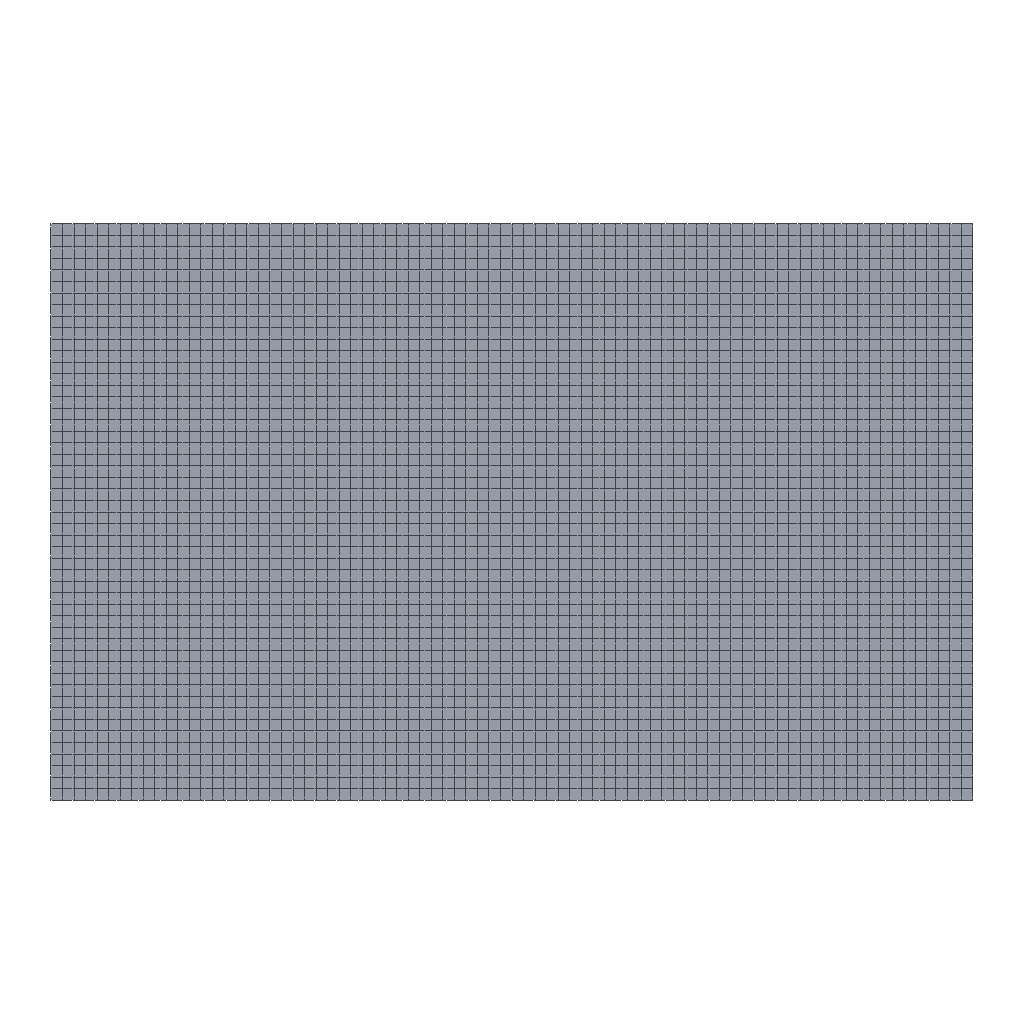Simulation study | abaqus
Set-up summary:
category,name,step,type,value,unit,region
solver,abaqus
solver,version,,,Abaqus/Standard 2020
units,not stated in the deck,,not stated
analysis,deck,,geostatic,geostatic
load_step,Step-1,Step-1,geostatic
load_step,Step-2,Step-2,soils
load_step,requested,,,2
mesh,nodes,,,4164
mesh,elements,,,4030
element_type,T2D2,,truss,30
element_type,CPE4P,,plane,4000
load,load commands in deck,,count,4
bc,support commands in deck,,count,3
material,CRACK,,in results
material,ROCK,,in results
check,setup vs results,,match,"per instance, exact: element labels, types and connectivity; labels of the nodes the elements use; coordinates of those nodes at SINGLE_PRECISION in 4 of 4 instance(s)"
Abaqus input file, long lists of numbers shortened:
*Heading
** Job name: Job-2 Model name: Model-1
** Generated by: Abaqus/CAE 2020
*Preprint, echo=NO, model=NO, history=NO, contact=NO
**
** PARTS
**
*Part, name=CRACK
*Node
      1,         -25.,          -4.
      2,         -25.,          -5.
** (9 more lines like these left out)
*Element, type=T2D2
 1,  1,  3
 2,  3,  4
** (8 more lines like these left out)
*Nset, nset=Set-1, generate
  1,  11,   1
*Elset, elset=Set-1, generate
  1,  10,   1
*Nset, nset=Set-4, generate
  1,  11,   1
*Elset, elset=Set-4, generate
  1,  10,   1
*Nset, nset=Set-5, generate
  1,  11,   1
*Elset, elset=Set-5, generate
  1,  10,   1
*Nset, nset=Set-14, generate
  1,  11,   1
*Elset, elset=Set-14, generate
  1,  10,   1
** Section: crack
*Solid Section, elset=Set-14, material=CRACK
1.,
*End Part
**
*Part, name=ROCK
*Node
      1,        58.75,        31.25
      2,        57.75,        31.25
** (4129 more lines like these left out)
*Element, type=CPE4P
   1,    1,    2,   83,   82
   2,    2,    3,   84,   83
** (3998 more lines like these left out)
*Nset, nset=Set-1, generate
    1,  4131,     1
*Elset, elset=Set-1, generate
    1,  4000,     1
** Section: rock
*Solid Section, elset=Set-1, material=rock
,
*End Part
**
**
** ASSEMBLY
**
*Assembly, name=Assembly
**
*Instance, name=CRACK-1, part=CRACK
       43.25,       -13.75,           0.
*End Instance
**
*Instance, name=ROCK-1, part=ROCK
*End Instance
**
*Instance, name=CRACK-2, part=CRACK
       38.25,       -13.75,           0.
*End Instance
**
*Instance, name=CRACK-3, part=CRACK
       48.25,       -13.75,           0.
*End Instance
**
*Nset, nset=Set-3, instance=CRACK-1, generate
  1,  11,   1
*Nset, nset=Set-3, instance=ROCK-1
    1,   81,   82,  162,  163,  243,  244,  324,  325,  405,  406,  486,  487,  567,  568,  648
  649,  729,  730,  810,  811,  891,  892,  972,  973, 1053, 1054, 1134, 1135, 1215, 1216, 1296
** (5 more lines like these left out)
*Elset, elset=Set-3, instance=CRACK-1, generate
  1,  10,   1
*Elset, elset=Set-3, instance=ROCK-1
    1,   80,   81,  160,  161,  240,  241,  320,  321,  400,  401,  480,  481,  560,  561,  640
  641,  720,  721,  800,  801,  880,  881,  960,  961, 1040, 1041, 1120, 1121, 1200, 1201, 1280
** (5 more lines like these left out)
*Nset, nset=Set-4, instance=CRACK-1, generate
  1,  11,   1
*Nset, nset=Set-4, instance=ROCK-1
    1,   81,   82,  162,  163,  243,  244,  324,  325,  405,  406,  486,  487,  567,  568,  648
  649,  729,  730,  810,  811,  891,  892,  972,  973, 1053, 1054, 1134, 1135, 1215, 1216, 1296
** (5 more lines like these left out)
*Elset, elset=Set-4, instance=CRACK-1, generate
  1,  10,   1
*Elset, elset=Set-4, instance=ROCK-1
    1,   80,   81,  160,  161,  240,  241,  320,  321,  400,  401,  480,  481,  560,  561,  640
  641,  720,  721,  800,  801,  880,  881,  960,  961, 1040, 1041, 1120, 1121, 1200, 1201, 1280
** (5 more lines like these left out)
*Nset, nset=Set-5, instance=ROCK-1
    1,   81,   82,  162,  163,  243,  244,  324,  325,  405,  406,  486,  487,  567,  568,  648
  649,  729,  730,  810,  811,  891,  892,  972,  973, 1053, 1054, 1134, 1135, 1215, 1216, 1296
** (5 more lines like these left out)
*Elset, elset=Set-5, instance=ROCK-1
    1,   80,   81,  160,  161,  240,  241,  320,  321,  400,  401,  480,  481,  560,  561,  640
  641,  720,  721,  800,  801,  880,  881,  960,  961, 1040, 1041, 1120, 1121, 1200, 1201, 1280
** (5 more lines like these left out)
*Nset, nset=Set-7, instance=CRACK-1, generate
  1,  11,   1
*Nset, nset=Set-7, instance=ROCK-1
    1,   81,   82,  162,  163,  243,  244,  324,  325,  405,  406,  486,  487,  567,  568,  648
  649,  729,  730,  810,  811,  891,  892,  972,  973, 1053, 1054, 1134, 1135, 1215, 1216, 1296
** (5 more lines like these left out)
*Elset, elset=Set-7, instance=CRACK-1, generate
  1,  10,   1
*Elset, elset=Set-7, instance=ROCK-1
    1,   80,   81,  160,  161,  240,  241,  320,  321,  400,  401,  480,  481,  560,  561,  640
  641,  720,  721,  800,  801,  880,  881,  960,  961, 1040, 1041, 1120, 1121, 1200, 1201, 1280
** (5 more lines like these left out)
*Nset, nset=Set-8, instance=ROCK-1
    1,   81,   82,  162,  163,  243,  244,  324,  325,  405,  406,  486,  487,  567,  568,  648
  649,  729,  730,  810,  811,  891,  892,  972,  973, 1053, 1054, 1134, 1135, 1215, 1216, 1296
** (5 more lines like these left out)
*Elset, elset=Set-8, instance=ROCK-1
    1,   80,   81,  160,  161,  240,  241,  320,  321,  400,  401,  480,  481,  560,  561,  640
  641,  720,  721,  800,  801,  880,  881,  960,  961, 1040, 1041, 1120, 1121, 1200, 1201, 1280
** (5 more lines like these left out)
*Nset, nset=Set-9, instance=ROCK-1, generate
    1,  4131,     1
*Elset, elset=Set-9, instance=ROCK-1, generate
    1,  4000,     1
*Nset, nset=Set-10, instance=ROCK-1
    1,    2,    3,    4,    5,    6,    7,    8,    9,   10,   11,   12,   13,   14,   15,   16
   17,   18,   19,   20,   21,   22,   23,   24,   25,   26,   27,   28,   29,   30,   31,   32
** (9 more lines like these left out)
*Elset, elset=Set-10, instance=ROCK-1
    1,    2,    3,    4,    5,    6,    7,    8,    9,   10,   11,   12,   13,   14,   15,   16
   17,   18,   19,   20,   21,   22,   23,   24,   25,   26,   27,   28,   29,   30,   31,   32
** (8 more lines like these left out)
*Nset, nset=Set-11, instance=CRACK-1, generate
  1,  11,   1
*Nset, nset=Set-11, instance=ROCK-1, generate
    1,  4131,     1
*Elset, elset=Set-11, instance=CRACK-1, generate
  1,  10,   1
*Elset, elset=Set-11, instance=ROCK-1, generate
    1,  4000,     1
*Nset, nset=Set-12, instance=CRACK-1, generate
  1,  11,   1
*Nset, nset=Set-12, instance=ROCK-1, generate
    1,  4131,     1
*Elset, elset=Set-12, instance=CRACK-1, generate
  1,  10,   1
*Elset, elset=Set-12, instance=ROCK-1, generate
    1,  4000,     1
*Nset, nset=Set-13, instance=ROCK-1
    1,    2,    3,    4,    5,    6,    7,    8,    9,   10,   11,   12,   13,   14,   15,   16
   17,   18,   19,   20,   21,   22,   23,   24,   25,   26,   27,   28,   29,   30,   31,   32
** (9 more lines like these left out)
*Elset, elset=Set-13, instance=ROCK-1
    1,    2,    3,    4,    5,    6,    7,    8,    9,   10,   11,   12,   13,   14,   15,   16
   17,   18,   19,   20,   21,   22,   23,   24,   25,   26,   27,   28,   29,   30,   31,   32
** (8 more lines like these left out)
*Nset, nset=Set-14, instance=ROCK-1
    1,    2,    3,    4,    5,    6,    7,    8,    9,   10,   11,   12,   13,   14,   15,   16
   17,   18,   19,   20,   21,   22,   23,   24,   25,   26,   27,   28,   29,   30,   31,   32
** (9 more lines like these left out)
*Elset, elset=Set-14, instance=ROCK-1
    1,    2,    3,    4,    5,    6,    7,    8,    9,   10,   11,   12,   13,   14,   15,   16
   17,   18,   19,   20,   21,   22,   23,   24,   25,   26,   27,   28,   29,   30,   31,   32
** (8 more lines like these left out)
*Nset, nset=Set-15, instance=ROCK-1, generate
  1,  81,   1
*Elset, elset=Set-15, instance=ROCK-1, generate
  1,  80,   1
*Nset, nset=Set-16, instance=ROCK-1
 4131,
*Nset, nset=Set-17, instance=CRACK-2
 2,
*Nset, nset=Set-18, instance=ROCK-1
 4131,
*Nset, nset=Set-19, instance=ROCK-1
    1,    2,    3,    4,    5,    6,    7,    8,    9,   10,   11,   12,   13,   14,   15,   16
   17,   18,   19,   20,   21,   22,   23,   24,   25,   26,   27,   28,   29,   30,   31,   32
** (9 more lines like these left out)
*Elset, elset=Set-19, instance=ROCK-1
    1,    2,    3,    4,    5,    6,    7,    8,    9,   10,   11,   12,   13,   14,   15,   16
   17,   18,   19,   20,   21,   22,   23,   24,   25,   26,   27,   28,   29,   30,   31,   32
** (8 more lines like these left out)
*Nset, nset=Set-20, instance=CRACK-1, generate
  1,  11,   1
*Nset, nset=Set-20, instance=ROCK-1, generate
    1,  4131,     1
*Nset, nset=Set-20, instance=CRACK-2, generate
  1,  11,   1
*Nset, nset=Set-20, instance=CRACK-3, generate
  1,  11,   1
*Elset, elset=Set-20, instance=CRACK-1, generate
  1,  10,   1
*Elset, elset=Set-20, instance=ROCK-1, generate
    1,  4000,     1
*Elset, elset=Set-20, instance=CRACK-2, generate
  1,  10,   1
*Elset, elset=Set-20, instance=CRACK-3, generate
  1,  10,   1
*Nset, nset=Set-21, instance=CRACK-2
 2,
*Nset, nset=Set-22, instance=ROCK-1
 4131,
*Nset, nset=_PickedSet16, internal, instance=ROCK-1, generate
    1,  4131,     1
*Elset, elset=_PickedSet16, internal, instance=ROCK-1, generate
    1,  4000,     1
*Nset, nset=_PickedSet28, internal, instance=CRACK-1, generate
  1,  11,   1
*Nset, nset=_PickedSet28, internal, instance=CRACK-2, generate
  1,  11,   1
*Nset, nset=_PickedSet28, internal, instance=CRACK-3, generate
  1,  11,   1
*Elset, elset=_PickedSet28, internal, instance=CRACK-1, generate
  1,  10,   1
*Elset, elset=_PickedSet28, internal, instance=CRACK-2, generate
  1,  10,   1
*Elset, elset=_PickedSet28, internal, instance=CRACK-3, generate
  1,  10,   1
*Elset, elset=_Surf-1_S3, internal, instance=ROCK-1, generate
 3921,  4000,     1
*Surface, type=ELEMENT, name=Surf-1
_Surf-1_S3, S3
*Elset, elset=_Surf-2_S3, internal, instance=ROCK-1, generate
 3921,  4000,     1
*Surface, type=ELEMENT, name=Surf-2
_Surf-2_S3, S3
*Elset, elset=_Surf-3_S3, internal, instance=ROCK-1, generate
 3921,  4000,     1
*Surface, type=ELEMENT, name=Surf-3
_Surf-3_S3, S3
*Elset, elset=_Surf-4_S3, internal, instance=ROCK-1, generate
 3921,  4000,     1
*Surface, type=ELEMENT, name=Surf-4
_Surf-4_S3, S3
*Elset, elset=_Surf-5_S3, internal, instance=ROCK-1, generate
 3921,  4000,     1
*Surface, type=ELEMENT, name=Surf-5
_Surf-5_S3, S3
*Elset, elset=_Surf-6_S3, internal, instance=ROCK-1, generate
 3921,  4000,     1
*Surface, type=ELEMENT, name=Surf-6
_Surf-6_S3, S3
*Nset, nset=Set-20_PP_, internal, instance=ROCK-1, generate
    1,  4131,     1
*Enrichment, name=Crack-1, type=PROPAGATION CRACK, elset=_PickedSet16, interaction=IntProp-1
*End Assembly
*Amplitude, name=Amp-1
             0.,              0.,             10.,             0.5,             20.,             0.8,             30.,              1.
            40.,              1.,             50.,              1.
*Amplitude, name=Amp-2
             0.,              0.,             10.,             0.3,             20.,             0.5,             30.,             0.7
            40.,             0.9,             50.,              1.
**
** MATERIALS
**
*Material, name=CRACK
*Elastic
 1e+10, 0.28
*Material, name=rock
*Damage Initiation, criterion=MAXPS
 2e+06,
*Damage Evolution, type=DISPLACEMENT, power=2.
 0.001,
*Damage Stabilization
0.0001
*Elastic
 2e+10, 0.2
*Fluid Leakoff
 5e-14, 1e-14
*Gap Flow
 0.001,
*Permeability, specific=9800.
 1e-08, 0.2
**
** INTERACTION PROPERTIES
**
*Surface Interaction, name=IntProp-1
1.,
*Friction, slip tolerance=0.005
 0.3,
*Surface Behavior, pressure-overclosure=HARD
*Initial Conditions, type=ENRICHMENT
ROCK-1.396, 1,Crack-1, 0.5, 0.
ROCK-1.396, 2,Crack-1, -0.5, 0.
ROCK-1.396, 3,Crack-1, -0.5, -1.
ROCK-1.396, 4,Crack-1, 0.5, -1.
ROCK-1.396, 1,Crack-1, 0.5, 0.
ROCK-1.396, 2,Crack-1, -0.5, 0.
ROCK-1.396, 3,Crack-1, -0.5, -1.
ROCK-1.396, 4,Crack-1, 0.5, -1.
ROCK-1.397, 1,Crack-1, 0.5, 0.
ROCK-1.397, 2,Crack-1, -0.5, 0.
ROCK-1.397, 3,Crack-1, -0.5, -1.
ROCK-1.397, 4,Crack-1, 0.5, -1.
**
** BOUNDARY CONDITIONS
**
** Name: BC-1 Type: 位移/转角
*Boundary
Set-5, 1, 1
** Name: BC-5 Type: 位移/转角
*Boundary
Set-14, 2, 2
**
** PREDEFINED FIELDS
**
** Name: Predefined Field-1   Type: Void ratio
*Initial Conditions, TYPE=RATIO
Set-11, 0.2
** Name: Predefined Field-3   Type: Stress
*Initial Conditions, type=STRESS
Set-9, -5e+06, -1e+07, 0., 0.,
** ----------------------------------------------------------------
**
** STEP: Step-1
**
*Step, name=Step-1, nlgeom=YES, unsymm=YES
*Geostatic
**
** OUTPUT REQUESTS
**
*Restart, write, frequency=0
**
** FIELD OUTPUT: F-Output-1
**
*Output, field
*Node Output
CF, PHILSM, POR, PSILSM, RF, U, V
*Element Output, directions=YES
FLVEL, LE, MISES, S, SAT, VOIDR
*Contact Output
CDISP, CSTRESS
**
** HISTORY OUTPUT: H-Output-1
**
*Output, history, variable=PRESELECT
*End Step
** ----------------------------------------------------------------
**
** STEP: Step-2
**
*Step, name=Step-2, nlgeom=YES, inc=100000, unsymm=YES
*Soils, consolidation, end=PERIOD, utol=1e+09, stabilize=0.0002, allsdtol=0.05, continue=NO
0.1, 50., 1e-07, 1.,
**
** BOUNDARY CONDITIONS
**
** Name: BC-6 Type: 孔隙压力
*Boundary
Set-20_PP_, 8, 8, 1e+07
**
** CONTROLS
**
*Controls, reset
*Controls, parameters=time incrementation
, , , , , , , 20, , ,
*cflow, amplitude=Amp-1, phantom=edge
ROCK-1.41, ROCK-1.41, -2e-3
*cflow, amplitude=Amp-2, phantom=edge
ROCK-1.409,ROCK-1.409, -2e-3
*cflow, amplitude=Amp-1, phantom=edge
ROCK-1.409, ROCK-1.409, -2e-3
**
** OUTPUT REQUESTS
**
*Restart, write, frequency=0
**
** FIELD OUTPUT: F-Output-1, F-Output-2
**
*Output, field
*Node Output
CF, PHILSM, POR, PSILSM, RF, U, V
*Element Output, directions=YES
FLVEL, LE, MISES, S, SAT, VOIDR
*Contact Output
CDISP, CSTRESS
**
** HISTORY OUTPUT: H-Output-1
**
*Output, history, variable=PRESELECT
*End Step
Results summary:
result,step,,completed,increments=1 time=1.0/1.0
result,step,,completed,increments=154 time=50.0/50.0
result,analysis,,,"soils, consolidation"
result,last_loadstep,,,2
result,primary field,,,"U, POR"
result,reaction total,,FX,3118.5,model units
result,reaction total,,FY,4747.0,model units
result,reaction total,,FZ,0.0,model units